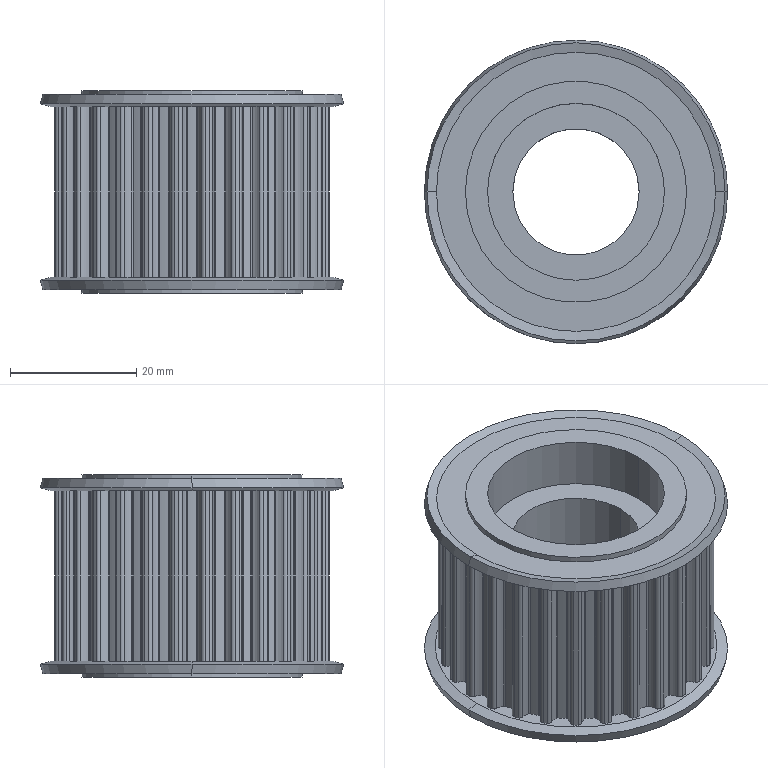Part | SolidWorks | features BaseBody 1 | 1 solid | 279 faces | box 48 x 48 x 32 mm | volume 29312 mm3 | cylinder 259 | cone 12 | plane 8 | commonest cylinder face diameters 1.1 x68 0.5 x64 6.55 x60 40.06 x29 43.6 x28 28 x4